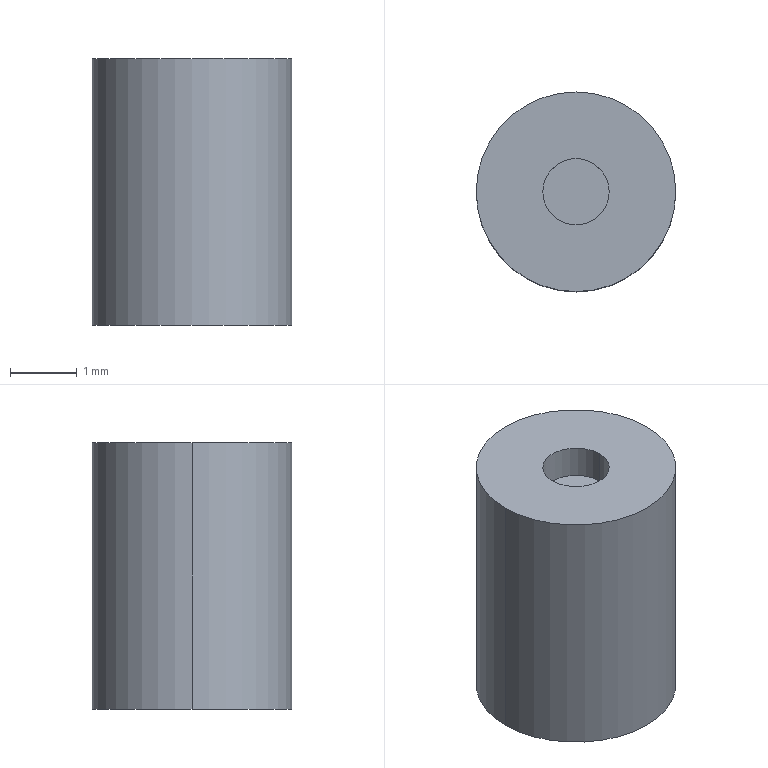Part | SolidWorks | features ICE 2, Extrusion 1 | 1 solid | 10 faces | box 3 x 3 x 4 mm | volume 27.685 mm3 | cylinder 6 | plane 4 | commonest cylinder face diameters 1 x4 3 x2
STEP:
#1=CARTESIAN_POINT('',(-276.031,-10.118,0.25));
#2=VERTEX_POINT('',#1);
#3=CARTESIAN_POINT('',(-277.031,-10.118,0.25));
#4=VERTEX_POINT('',#3);
#5=CARTESIAN_POINT('',(-276.531,-10.118,0.25));
#6=DIRECTION('',(0.,0.,-1.));
#7=DIRECTION('',(-1.,0.,0.));
#8=AXIS2_PLACEMENT_3D('',#5,#6,#7);
#9=CIRCLE('',#8,0.5);
#10=EDGE_CURVE('',#2,#4,#9,.T.);
#11=ORIENTED_EDGE('',*,*,#10,.F.);
#12=CARTESIAN_POINT('',(-276.031,-10.118,0.));
#13=VERTEX_POINT('',#12);
#14=CARTESIAN_POINT('',(-276.031,-10.118,0.25));
#15=DIRECTION('',(0.,0.,-1.));
#16=VECTOR('',#15,1000.);
#17=LINE('',#14,#16);
#18=EDGE_CURVE('',#2,#13,#17,.T.);
#19=ORIENTED_EDGE('',*,*,#18,.T.);
#20=CARTESIAN_POINT('',(-277.031,-10.118,0.));
#21=VERTEX_POINT('',#20);
#22=CARTESIAN_POINT('',(-276.531,-10.118,0.));
#23=DIRECTION('',(0.,0.,-1.));
#24=DIRECTION('',(-1.,0.,0.));
#25=AXIS2_PLACEMENT_3D('',#22,#23,#24);
#26=CIRCLE('',#25,0.5);
#27=EDGE_CURVE('',#13,#21,#26,.T.);
#28=ORIENTED_EDGE('',*,*,#27,.T.);
#29=CARTESIAN_POINT('',(-277.031,-10.118,0.25));
#30=DIRECTION('',(0.,0.,-1.));
#31=VECTOR('',#30,1000.);
#32=LINE('',#29,#31);
#33=EDGE_CURVE('',#4,#21,#32,.T.);
#34=ORIENTED_EDGE('',*,*,#33,.F.);
#35=EDGE_LOOP('',(#11,#19,#28,#34));
#36=FACE_OUTER_BOUND('',#35,.T.);
#37=CARTESIAN_POINT('',(-276.531,-10.118,0.25));
#38=DIRECTION('',(0.,0.,-1.));
#39=DIRECTION('',(-1.,0.,0.));
#40=AXIS2_PLACEMENT_3D('',#37,#38,#39);
#41=CYLINDRICAL_SURFACE('',#40,0.5);
#42=ADVANCED_FACE('',(#36),#41,.F.);
#43=CARTESIAN_POINT('',(-277.031,-10.118,3.5));
#44=VERTEX_POINT('',#43);
#45=CARTESIAN_POINT('',(-276.031,-10.118,3.5));
#46=VERTEX_POINT('',#45);
#47=CARTESIAN_POINT('',(-276.531,-10.118,3.5));
#48=DIRECTION('',(0.,0.,1.));
#49=DIRECTION('',(1.,0.,0.));
#50=AXIS2_PLACEMENT_3D('',#47,#48,#49);
#51=CIRCLE('',#50,0.5);
#52=EDGE_CURVE('',#44,#46,#51,.T.);
#53=ORIENTED_EDGE('',*,*,#52,.F.);
#54=CARTESIAN_POINT('',(-277.031,-10.118,4.));
#55=VERTEX_POINT('',#54);
#56=CARTESIAN_POINT('',(-277.031,-10.118,3.5));
#57=DIRECTION('',(0.,0.,1.));
#58=VECTOR('',#57,1000.);
#59=LINE('',#56,#58);
#60=EDGE_CURVE('',#44,#55,#59,.T.);
#61=ORIENTED_EDGE('',*,*,#60,.T.);
#62=CARTESIAN_POINT('',(-276.031,-10.118,4.));
#63=VERTEX_POINT('',#62);
#64=CARTESIAN_POINT('',(-276.531,-10.118,4.));
#65=DIRECTION('',(0.,0.,1.));
#66=DIRECTION('',(1.,0.,0.));
#67=AXIS2_PLACEMENT_3D('',#64,#65,#66);
#68=CIRCLE('',#67,0.5);
#69=EDGE_CURVE('',#55,#63,#68,.T.);
#70=ORIENTED_EDGE('',*,*,#69,.T.);
#71=CARTESIAN_POINT('',(-276.031,-10.118,3.5));
#72=DIRECTION('',(0.,0.,1.));
#73=VECTOR('',#72,1000.);
#74=LINE('',#71,#73);
#75=EDGE_CURVE('',#46,#63,#74,.T.);
#76=ORIENTED_EDGE('',*,*,#75,.F.);
#77=EDGE_LOOP('',(#53,#61,#70,#76));
#78=FACE_OUTER_BOUND('',#77,.T.);
#79=CARTESIAN_POINT('',(-276.531,-10.118,3.5));
#80=DIRECTION('',(0.,0.,1.));
#81=DIRECTION('',(1.,0.,0.));
#82=AXIS2_PLACEMENT_3D('',#79,#80,#81);
#83=CYLINDRICAL_SURFACE('',#82,0.5);
#84=ADVANCED_FACE('',(#78),#83,.F.);
#85=CARTESIAN_POINT('',(-275.031,-10.118,4.));
#86=VERTEX_POINT('',#85);
#87=CARTESIAN_POINT('',(-278.031,-10.118,4.));
#88=VERTEX_POINT('',#87);
#89=CARTESIAN_POINT('',(-276.531,-10.118,4.));
#90=DIRECTION('',(0.,0.,1.));
#91=DIRECTION('',(1.,0.,0.));
#92=AXIS2_PLACEMENT_3D('',#89,#90,#91);
#93=CIRCLE('',#92,1.5);
#94=EDGE_CURVE('',#86,#88,#93,.T.);
#95=ORIENTED_EDGE('',*,*,#94,.F.);
#96=CARTESIAN_POINT('',(-275.031,-10.118,0.));
#97=VERTEX_POINT('',#96);
#98=CARTESIAN_POINT('',(-275.031,-10.118,4.));
#99=DIRECTION('',(0.,0.,-1.));
#100=VECTOR('',#99,1000.);
#101=LINE('',#98,#100);
#102=EDGE_CURVE('',#86,#97,#101,.T.);
#103=ORIENTED_EDGE('',*,*,#102,.T.);
#104=CARTESIAN_POINT('',(-278.031,-10.118,0.));
#105=VERTEX_POINT('',#104);
#106=CARTESIAN_POINT('',(-276.531,-10.118,0.));
#107=DIRECTION('',(0.,0.,1.));
#108=DIRECTION('',(1.,0.,0.));
#109=AXIS2_PLACEMENT_3D('',#106,#107,#108);
#110=CIRCLE('',#109,1.5);
#111=EDGE_CURVE('',#97,#105,#110,.T.);
#112=ORIENTED_EDGE('',*,*,#111,.T.);
#113=CARTESIAN_POINT('',(-278.031,-10.118,4.));
#114=DIRECTION('',(0.,0.,-1.));
#115=VECTOR('',#114,1000.);
#116=LINE('',#113,#115);
#117=EDGE_CURVE('',#88,#105,#116,.T.);
#118=ORIENTED_EDGE('',*,*,#117,.F.);
#119=EDGE_LOOP('',(#95,#103,#112,#118));
#120=FACE_OUTER_BOUND('',#119,.T.);
#121=CARTESIAN_POINT('',(-276.531,-10.118,4.));
#122=DIRECTION('',(0.,0.,-1.));
#123=DIRECTION('',(-1.,0.,0.));
#124=AXIS2_PLACEMENT_3D('',#121,#122,#123);
#125=CYLINDRICAL_SURFACE('',#124,1.5);
#126=ADVANCED_FACE('',(#120),#125,.T.);
#127=ORIENTED_EDGE('',*,*,#102,.F.);
#128=CARTESIAN_POINT('',(-276.531,-10.118,4.));
#129=DIRECTION('',(0.,0.,1.));
#130=DIRECTION('',(1.,0.,0.));
#131=AXIS2_PLACEMENT_3D('',#128,#129,#130);
#132=CIRCLE('',#131,1.5);
#133=EDGE_CURVE('',#88,#86,#132,.T.);
#134=ORIENTED_EDGE('',*,*,#133,.F.);
#135=ORIENTED_EDGE('',*,*,#117,.T.);
#136=CARTESIAN_POINT('',(-276.531,-10.118,0.));
#137=DIRECTION('',(0.,0.,1.));
#138=DIRECTION('',(1.,0.,0.));
#139=AXIS2_PLACEMENT_3D('',#136,#137,#138);
#140=CIRCLE('',#139,1.5);
#141=EDGE_CURVE('',#105,#97,#140,.T.);
#142=ORIENTED_EDGE('',*,*,#141,.T.);
#143=EDGE_LOOP('',(#127,#134,#135,#142));
#144=FACE_OUTER_BOUND('',#143,.T.);
#145=CARTESIAN_POINT('',(-276.531,-10.118,4.));
#146=DIRECTION('',(0.,0.,-1.));
#147=DIRECTION('',(-1.,0.,0.));
#148=AXIS2_PLACEMENT_3D('',#145,#146,#147);
#149=CYLINDRICAL_SURFACE('',#148,1.5);
#150=ADVANCED_FACE('',(#144),#149,.T.);
#151=CARTESIAN_POINT('',(-276.531,-10.118,4.));
#152=DIRECTION('',(0.,0.,1.));
#153=DIRECTION('',(1.,0.,0.));
#154=AXIS2_PLACEMENT_3D('',#151,#152,#153);
#155=CIRCLE('',#154,0.5);
#156=EDGE_CURVE('',#63,#55,#155,.T.);
#157=ORIENTED_EDGE('',*,*,#156,.F.);
#158=ORIENTED_EDGE('',*,*,#69,.F.);
#159=EDGE_LOOP('',(#157,#158));
#160=FACE_BOUND('',#159,.T.);
#161=ORIENTED_EDGE('',*,*,#133,.T.);
#162=ORIENTED_EDGE('',*,*,#94,.T.);
#163=EDGE_LOOP('',(#161,#162));
#164=FACE_OUTER_BOUND('',#163,.T.);
#165=CARTESIAN_POINT('',(-276.531,-10.118,4.));
#166=DIRECTION('',(0.,0.,1.));
#167=DIRECTION('',(1.,0.,0.));
#168=AXIS2_PLACEMENT_3D('',#165,#166,#167);
#169=PLANE('',#168);
#170=ADVANCED_FACE('',(#160,#164),#169,.T.);
#171=CARTESIAN_POINT('',(-276.531,-10.118,0.));
#172=DIRECTION('',(0.,0.,-1.));
#173=DIRECTION('',(-1.,0.,0.));
#174=AXIS2_PLACEMENT_3D('',#171,#172,#173);
#175=CIRCLE('',#174,0.5);
#176=EDGE_CURVE('',#21,#13,#175,.T.);
#177=ORIENTED_EDGE('',*,*,#176,.F.);
#178=ORIENTED_EDGE('',*,*,#27,.F.);
#179=EDGE_LOOP('',(#177,#178));
#180=FACE_BOUND('',#179,.T.);
#181=ORIENTED_EDGE('',*,*,#141,.F.);
#182=ORIENTED_EDGE('',*,*,#111,.F.);
#183=EDGE_LOOP('',(#181,#182));
#184=FACE_OUTER_BOUND('',#183,.T.);
#185=CARTESIAN_POINT('',(-276.531,-10.118,0.));
#186=DIRECTION('',(0.,0.,1.));
#187=DIRECTION('',(1.,0.,0.));
#188=AXIS2_PLACEMENT_3D('',#185,#186,#187);
#189=PLANE('',#188);
#190=ADVANCED_FACE('',(#180,#184),#189,.F.);
#191=ORIENTED_EDGE('',*,*,#60,.F.);
#192=CARTESIAN_POINT('',(-276.531,-10.118,3.5));
#193=DIRECTION('',(0.,0.,1.));
#194=DIRECTION('',(1.,0.,0.));
#195=AXIS2_PLACEMENT_3D('',#192,#193,#194);
#196=CIRCLE('',#195,0.5);
#197=EDGE_CURVE('',#46,#44,#196,.T.);
#198=ORIENTED_EDGE('',*,*,#197,.F.);
#199=ORIENTED_EDGE('',*,*,#75,.T.);
#200=ORIENTED_EDGE('',*,*,#156,.T.);
#201=EDGE_LOOP('',(#191,#198,#199,#200));
#202=FACE_OUTER_BOUND('',#201,.T.);
#203=CARTESIAN_POINT('',(-276.531,-10.118,3.5));
#204=DIRECTION('',(0.,0.,1.));
#205=DIRECTION('',(1.,0.,0.));
#206=AXIS2_PLACEMENT_3D('',#203,#204,#205);
#207=CYLINDRICAL_SURFACE('',#206,0.5);
#208=ADVANCED_FACE('',(#202),#207,.F.);
#209=ORIENTED_EDGE('',*,*,#197,.T.);
#210=ORIENTED_EDGE('',*,*,#52,.T.);
#211=EDGE_LOOP('',(#209,#210));
#212=FACE_OUTER_BOUND('',#211,.T.);
#213=CARTESIAN_POINT('',(-276.531,-10.118,3.5));
#214=DIRECTION('',(0.,0.,1.));
#215=DIRECTION('',(1.,0.,0.));
#216=AXIS2_PLACEMENT_3D('',#213,#214,#215);
#217=PLANE('',#216);
#218=ADVANCED_FACE('',(#212),#217,.T.);
#219=ORIENTED_EDGE('',*,*,#18,.F.);
#220=CARTESIAN_POINT('',(-276.531,-10.118,0.25));
#221=DIRECTION('',(0.,0.,-1.));
#222=DIRECTION('',(-1.,0.,0.));
#223=AXIS2_PLACEMENT_3D('',#220,#221,#222);
#224=CIRCLE('',#223,0.5);
#225=EDGE_CURVE('',#4,#2,#224,.T.);
#226=ORIENTED_EDGE('',*,*,#225,.F.);
#227=ORIENTED_EDGE('',*,*,#33,.T.);
#228=ORIENTED_EDGE('',*,*,#176,.T.);
#229=EDGE_LOOP('',(#219,#226,#227,#228));
#230=FACE_OUTER_BOUND('',#229,.T.);
#231=CARTESIAN_POINT('',(-276.531,-10.118,0.25));
#232=DIRECTION('',(0.,0.,-1.));
#233=DIRECTION('',(-1.,0.,0.));
#234=AXIS2_PLACEMENT_3D('',#231,#232,#233);
#235=CYLINDRICAL_SURFACE('',#234,0.5);
#236=ADVANCED_FACE('',(#230),#235,.F.);
#237=ORIENTED_EDGE('',*,*,#225,.T.);
#238=ORIENTED_EDGE('',*,*,#10,.T.);
#239=EDGE_LOOP('',(#237,#238));
#240=FACE_OUTER_BOUND('',#239,.T.);
#241=CARTESIAN_POINT('',(-276.531,-10.118,0.25));
#242=DIRECTION('',(0.,0.,-1.));
#243=DIRECTION('',(-1.,0.,0.));
#244=AXIS2_PLACEMENT_3D('',#241,#242,#243);
#245=PLANE('',#244);
#246=ADVANCED_FACE('',(#240),#245,.T.);
#247=CLOSED_SHELL('',(#42,#84,#126,#150,#170,#190,#208,#218,#236,#246));
#248=MANIFOLD_SOLID_BREP('',#247);
#249=CARTESIAN_POINT('',(0.,0.,0.));
#250=DIRECTION('',(0.,0.,1.));
#251=DIRECTION('',(1.,0.,0.));
#252=AXIS2_PLACEMENT_3D('',#249,#250,#251);
#253=(LENGTH_UNIT()NAMED_UNIT(*)SI_UNIT(.MILLI.,.METRE.));
#254=UNCERTAINTY_MEASURE_WITH_UNIT(LENGTH_MEASURE(0.00001),#253,'','');
#255=(NAMED_UNIT(*)PLANE_ANGLE_UNIT()SI_UNIT($,.RADIAN.));
#256=(NAMED_UNIT(*)SI_UNIT($,.STERADIAN.)SOLID_ANGLE_UNIT());
#257=(GEOMETRIC_REPRESENTATION_CONTEXT(3)GLOBAL_UNCERTAINTY_ASSIGNED_CONTEXT((#254))GLOBAL_UNIT_ASSIGNED_CONTEXT((#253,#255,#256))REPRESENTATION_CONTEXT('',''));
#258=ADVANCED_BREP_SHAPE_REPRESENTATION('',(#248,#252),#257);